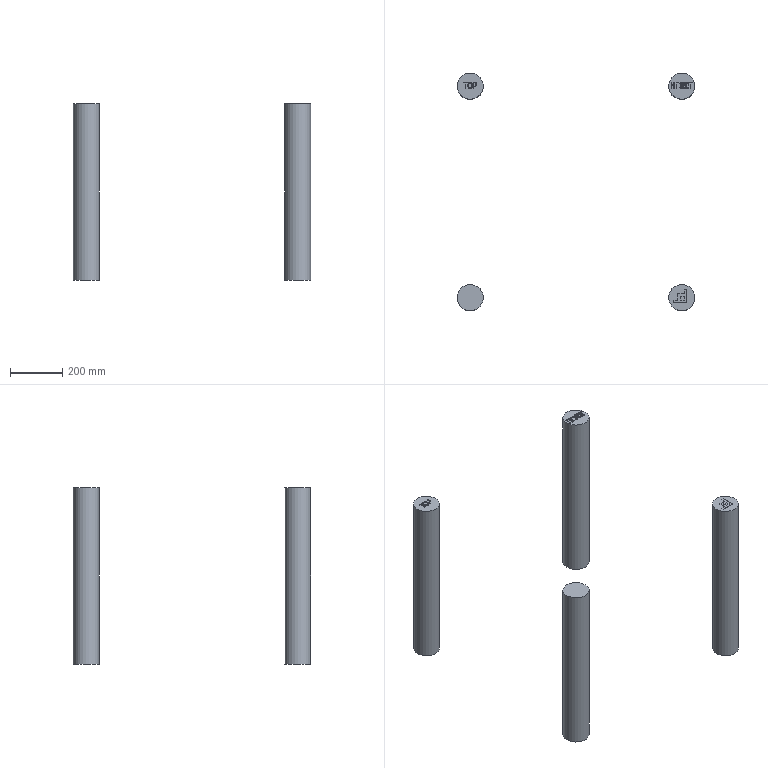Part | STEP file | Tie Bars 360T | 4 solids | 106 faces | box 910 x 910 x 677 mm | volume 21266346 mm3 | plane 79 | other 23 | cylinder 4 | commonest cylinder face diameters 100 x4